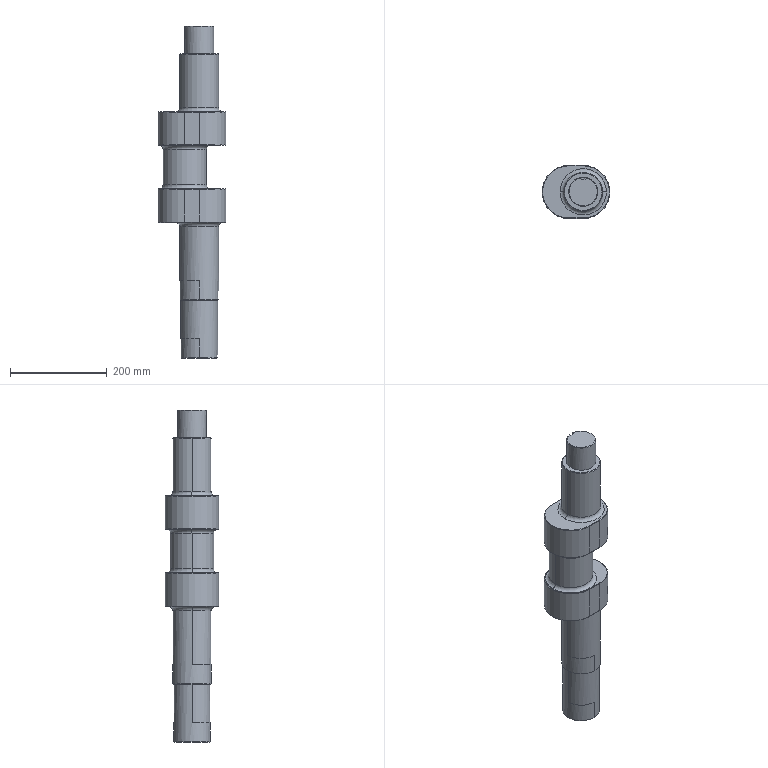Part | Creo | features PROTRUSION 9, CURVE 8, DATUM PLANE 3, CHAMFER 2, MIRROR 2, ROUND 2, COORDINATE SYSTEM 1, CUT 1 | 1 solid | 61 faces | box 140 x 110 x 687 mm | volume 4490252 mm3 | plane 23 | cylinder 15 | cone 15 | torus 8 | commonest cylinder face diameters 80 x4 110 x4 60 x2 76 x2 90 x2 8 x1